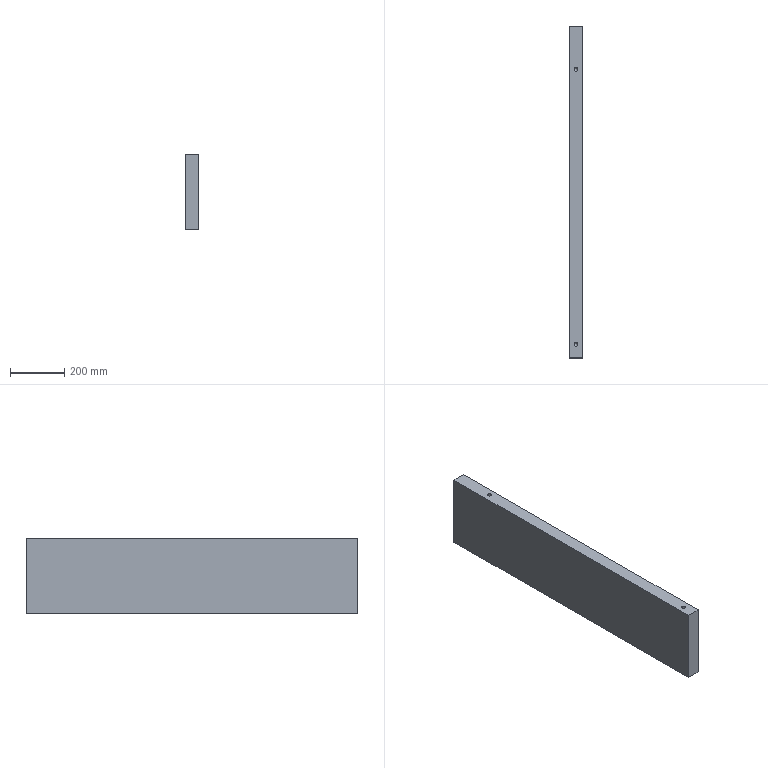Part | NX | features 29 2 | 1 solid | 16 faces | box 50 x 1225 x 280.5 mm | volume 17149943 mm3 | plane 6 | cylinder 5 | cone 5 | commonest cylinder face diameters 14.1 x5
STEP:
#1=CARTESIAN_POINT('',(2700.05,512.5,-493.5));
#2=VERTEX_POINT('',#1);
#3=CARTESIAN_POINT('',(2693.,512.5,-493.5));
#4=DIRECTION('',(0.,0.,1.));
#5=DIRECTION('',(1.,0.,0.));
#6=AXIS2_PLACEMENT_3D('',#3,#4,#5);
#7=CIRCLE('',#6,7.05);
#8=EDGE_CURVE('',#2,#2,#7,.T.);
#9=ORIENTED_EDGE('',*,*,#8,.T.);
#10=EDGE_LOOP('',(#9));
#11=FACE_BOUND('',#10,.T.);
#12=CARTESIAN_POINT('',(2668.,-552.5,-493.5));
#13=VERTEX_POINT('',#12);
#14=CARTESIAN_POINT('',(2718.,-552.5,-493.5));
#15=VERTEX_POINT('',#14);
#16=CARTESIAN_POINT('',(275.5,-552.5,-493.5));
#17=DIRECTION('',(1.,0.,0.));
#18=VECTOR('',#17,1000.);
#19=LINE('',#16,#18);
#20=EDGE_CURVE('',#13,#15,#19,.T.);
#21=ORIENTED_EDGE('',*,*,#20,.F.);
#22=CARTESIAN_POINT('',(2668.,672.5,-493.5));
#23=VERTEX_POINT('',#22);
#24=CARTESIAN_POINT('',(2668.,193.,-493.5));
#25=DIRECTION('',(0.,-1.,0.));
#26=VECTOR('',#25,1000.);
#27=LINE('',#24,#26);
#28=EDGE_CURVE('',#23,#13,#27,.T.);
#29=ORIENTED_EDGE('',*,*,#28,.F.);
#30=CARTESIAN_POINT('',(2718.,672.5,-493.5));
#31=VERTEX_POINT('',#30);
#32=CARTESIAN_POINT('',(275.5,672.5,-493.5));
#33=DIRECTION('',(1.,0.,0.));
#34=VECTOR('',#33,1000.);
#35=LINE('',#32,#34);
#36=EDGE_CURVE('',#23,#31,#35,.T.);
#37=ORIENTED_EDGE('',*,*,#36,.T.);
#38=CARTESIAN_POINT('',(2718.,193.,-493.5));
#39=DIRECTION('',(0.,1.,0.));
#40=VECTOR('',#39,1000.);
#41=LINE('',#38,#40);
#42=EDGE_CURVE('',#15,#31,#41,.T.);
#43=ORIENTED_EDGE('',*,*,#42,.F.);
#44=EDGE_LOOP('',(#21,#29,#37,#43));
#45=FACE_BOUND('',#44,.T.);
#46=CARTESIAN_POINT('',(2700.05,-502.5,-493.5));
#47=VERTEX_POINT('',#46);
#48=CARTESIAN_POINT('',(2693.,-502.5,-493.5));
#49=DIRECTION('',(0.,0.,1.));
#50=DIRECTION('',(1.,0.,0.));
#51=AXIS2_PLACEMENT_3D('',#48,#49,#50);
#52=CIRCLE('',#51,7.05);
#53=EDGE_CURVE('',#47,#47,#52,.T.);
#54=ORIENTED_EDGE('',*,*,#53,.T.);
#55=EDGE_LOOP('',(#54));
#56=FACE_BOUND('',#55,.T.);
#57=CARTESIAN_POINT('',(2700.05,60.,-493.5));
#58=VERTEX_POINT('',#57);
#59=CARTESIAN_POINT('',(2693.,60.,-493.5));
#60=DIRECTION('',(0.,0.,1.));
#61=DIRECTION('',(1.,0.,0.));
#62=AXIS2_PLACEMENT_3D('',#59,#60,#61);
#63=CIRCLE('',#62,7.05);
#64=EDGE_CURVE('',#58,#58,#63,.T.);
#65=ORIENTED_EDGE('',*,*,#64,.T.);
#66=EDGE_LOOP('',(#65));
#67=FACE_BOUND('',#66,.T.);
#68=CARTESIAN_POINT('',(2238.,0.,-493.5));
#69=DIRECTION('',(0.,0.,-1.));
#70=DIRECTION('',(1.,0.,0.));
#71=AXIS2_PLACEMENT_3D('',#68,#69,#70);
#72=PLANE('',#71);
#73=ADVANCED_FACE('',(#11,#45,#56,#67),#72,.T.);
#74=CARTESIAN_POINT('',(2700.05,512.5,-213.));
#75=VERTEX_POINT('',#74);
#76=CARTESIAN_POINT('',(2693.,512.5,-213.));
#77=DIRECTION('',(0.,0.,-1.));
#78=DIRECTION('',(1.,0.,0.));
#79=AXIS2_PLACEMENT_3D('',#76,#77,#78);
#80=CIRCLE('',#79,7.05);
#81=EDGE_CURVE('',#75,#75,#80,.T.);
#82=ORIENTED_EDGE('',*,*,#81,.T.);
#83=EDGE_LOOP('',(#82));
#84=FACE_BOUND('',#83,.T.);
#85=CARTESIAN_POINT('',(2718.,-552.5,-213.));
#86=VERTEX_POINT('',#85);
#87=CARTESIAN_POINT('',(2668.,-552.5,-213.));
#88=VERTEX_POINT('',#87);
#89=CARTESIAN_POINT('',(275.5,-552.5,-213.));
#90=DIRECTION('',(-1.,0.,0.));
#91=VECTOR('',#90,1000.);
#92=LINE('',#89,#91);
#93=EDGE_CURVE('',#86,#88,#92,.T.);
#94=ORIENTED_EDGE('',*,*,#93,.F.);
#95=CARTESIAN_POINT('',(2718.,672.5,-213.));
#96=VERTEX_POINT('',#95);
#97=CARTESIAN_POINT('',(2718.,193.,-213.));
#98=DIRECTION('',(0.,-1.,0.));
#99=VECTOR('',#98,1000.);
#100=LINE('',#97,#99);
#101=EDGE_CURVE('',#96,#86,#100,.T.);
#102=ORIENTED_EDGE('',*,*,#101,.F.);
#103=CARTESIAN_POINT('',(2668.,672.5,-213.));
#104=VERTEX_POINT('',#103);
#105=CARTESIAN_POINT('',(275.5,672.5,-213.));
#106=DIRECTION('',(-1.,0.,0.));
#107=VECTOR('',#106,1000.);
#108=LINE('',#105,#107);
#109=EDGE_CURVE('',#96,#104,#108,.T.);
#110=ORIENTED_EDGE('',*,*,#109,.T.);
#111=CARTESIAN_POINT('',(2668.,193.,-213.));
#112=DIRECTION('',(0.,1.,0.));
#113=VECTOR('',#112,1000.);
#114=LINE('',#111,#113);
#115=EDGE_CURVE('',#88,#104,#114,.T.);
#116=ORIENTED_EDGE('',*,*,#115,.F.);
#117=EDGE_LOOP('',(#94,#102,#110,#116));
#118=FACE_BOUND('',#117,.T.);
#119=CARTESIAN_POINT('',(2700.05,-502.5,-213.));
#120=VERTEX_POINT('',#119);
#121=CARTESIAN_POINT('',(2693.,-502.5,-213.));
#122=DIRECTION('',(0.,0.,-1.));
#123=DIRECTION('',(1.,0.,0.));
#124=AXIS2_PLACEMENT_3D('',#121,#122,#123);
#125=CIRCLE('',#124,7.05);
#126=EDGE_CURVE('',#120,#120,#125,.T.);
#127=ORIENTED_EDGE('',*,*,#126,.T.);
#128=EDGE_LOOP('',(#127));
#129=FACE_BOUND('',#128,.T.);
#130=CARTESIAN_POINT('',(2238.,0.,-213.));
#131=DIRECTION('',(0.,0.,1.));
#132=DIRECTION('',(-1.,0.,0.));
#133=AXIS2_PLACEMENT_3D('',#130,#131,#132);
#134=PLANE('',#133);
#135=ADVANCED_FACE('',(#84,#118,#129),#134,.T.);
#136=CARTESIAN_POINT('',(2668.,-552.5,-205.5));
#137=DIRECTION('',(0.,0.,1.));
#138=VECTOR('',#137,1000.);
#139=LINE('',#136,#138);
#140=EDGE_CURVE('',#13,#88,#139,.T.);
#141=ORIENTED_EDGE('',*,*,#140,.F.);
#142=ORIENTED_EDGE('',*,*,#20,.T.);
#143=CARTESIAN_POINT('',(2718.,-552.5,-205.5));
#144=DIRECTION('',(0.,0.,-1.));
#145=VECTOR('',#144,1000.);
#146=LINE('',#143,#145);
#147=EDGE_CURVE('',#86,#15,#146,.T.);
#148=ORIENTED_EDGE('',*,*,#147,.F.);
#149=ORIENTED_EDGE('',*,*,#93,.T.);
#150=EDGE_LOOP('',(#141,#142,#148,#149));
#151=FACE_BOUND('',#150,.T.);
#152=CARTESIAN_POINT('',(275.5,-552.5,-113.));
#153=DIRECTION('',(0.,1.,0.));
#154=DIRECTION('',(1.,0.,0.));
#155=AXIS2_PLACEMENT_3D('',#152,#153,#154);
#156=PLANE('',#155);
#157=ADVANCED_FACE('',(#151),#156,.F.);
#158=CARTESIAN_POINT('',(2668.,672.5,-205.5));
#159=DIRECTION('',(0.,0.,1.));
#160=VECTOR('',#159,1000.);
#161=LINE('',#158,#160);
#162=EDGE_CURVE('',#23,#104,#161,.T.);
#163=ORIENTED_EDGE('',*,*,#162,.F.);
#164=ORIENTED_EDGE('',*,*,#28,.T.);
#165=ORIENTED_EDGE('',*,*,#140,.T.);
#166=ORIENTED_EDGE('',*,*,#115,.T.);
#167=EDGE_LOOP('',(#163,#164,#165,#166));
#168=FACE_BOUND('',#167,.T.);
#169=CARTESIAN_POINT('',(2668.,193.,-205.5));
#170=DIRECTION('',(-1.,0.,0.));
#171=DIRECTION('',(0.,0.,1.));
#172=AXIS2_PLACEMENT_3D('',#169,#170,#171);
#173=PLANE('',#172);
#174=ADVANCED_FACE('',(#168),#173,.T.);
#175=ORIENTED_EDGE('',*,*,#147,.T.);
#176=ORIENTED_EDGE('',*,*,#42,.T.);
#177=CARTESIAN_POINT('',(2718.,672.5,91.));
#178=DIRECTION('',(0.,0.,1.));
#179=VECTOR('',#178,1000.);
#180=LINE('',#177,#179);
#181=EDGE_CURVE('',#31,#96,#180,.T.);
#182=ORIENTED_EDGE('',*,*,#181,.T.);
#183=ORIENTED_EDGE('',*,*,#101,.T.);
#184=EDGE_LOOP('',(#175,#176,#182,#183));
#185=FACE_BOUND('',#184,.T.);
#186=CARTESIAN_POINT('',(2718.,193.,-205.5));
#187=DIRECTION('',(1.,0.,0.));
#188=DIRECTION('',(0.,0.,-1.));
#189=AXIS2_PLACEMENT_3D('',#186,#187,#188);
#190=PLANE('',#189);
#191=ADVANCED_FACE('',(#185),#190,.T.);
#192=ORIENTED_EDGE('',*,*,#36,.F.);
#193=ORIENTED_EDGE('',*,*,#162,.T.);
#194=ORIENTED_EDGE('',*,*,#109,.F.);
#195=ORIENTED_EDGE('',*,*,#181,.F.);
#196=EDGE_LOOP('',(#192,#193,#194,#195));
#197=FACE_BOUND('',#196,.T.);
#198=CARTESIAN_POINT('',(275.5,672.5,91.));
#199=DIRECTION('',(0.,-1.,0.));
#200=DIRECTION('',(-1.,0.,0.));
#201=AXIS2_PLACEMENT_3D('',#198,#199,#200);
#202=PLANE('',#201);
#203=ADVANCED_FACE('',(#197),#202,.F.);
#204=CARTESIAN_POINT('',(2685.95,512.5,-249.95));
#205=VERTEX_POINT('',#204);
#206=CARTESIAN_POINT('',(2693.,512.5,-249.95));
#207=DIRECTION('',(0.,0.,-1.));
#208=DIRECTION('',(-1.,0.,0.));
#209=AXIS2_PLACEMENT_3D('',#206,#207,#208);
#210=CIRCLE('',#209,7.05);
#211=EDGE_CURVE('',#205,#205,#210,.T.);
#212=ORIENTED_EDGE('',*,*,#211,.T.);
#213=EDGE_LOOP('',(#212));
#214=FACE_BOUND('',#213,.T.);
#215=ORIENTED_EDGE('',*,*,#81,.F.);
#216=EDGE_LOOP('',(#215));
#217=FACE_BOUND('',#216,.T.);
#218=CARTESIAN_POINT('',(2693.,512.5,-213.));
#219=DIRECTION('',(0.,0.,-1.));
#220=DIRECTION('',(-1.,0.,0.));
#221=AXIS2_PLACEMENT_3D('',#218,#219,#220);
#222=CYLINDRICAL_SURFACE('',#221,7.05);
#223=ADVANCED_FACE('',(#214,#217),#222,.F.);
#224=CARTESIAN_POINT('',(2693.,512.5,-257.));
#225=VERTEX_POINT('',#224);
#226=VERTEX_LOOP('',#225);
#227=FACE_BOUND('',#226,.T.);
#228=ORIENTED_EDGE('',*,*,#211,.F.);
#229=EDGE_LOOP('',(#228));
#230=FACE_BOUND('',#229,.T.);
#231=CARTESIAN_POINT('',(2693.,512.5,-249.95));
#232=DIRECTION('',(0.,0.,1.));
#233=DIRECTION('',(-1.,0.,0.));
#234=AXIS2_PLACEMENT_3D('',#231,#232,#233);
#235=CONICAL_SURFACE('',#234,7.05,0.7854);
#236=ADVANCED_FACE('',(#227,#230),#235,.F.);
#237=CARTESIAN_POINT('',(2685.95,-502.5,-249.95));
#238=VERTEX_POINT('',#237);
#239=CARTESIAN_POINT('',(2693.,-502.5,-249.95));
#240=DIRECTION('',(0.,0.,-1.));
#241=DIRECTION('',(-1.,0.,0.));
#242=AXIS2_PLACEMENT_3D('',#239,#240,#241);
#243=CIRCLE('',#242,7.05);
#244=EDGE_CURVE('',#238,#238,#243,.T.);
#245=ORIENTED_EDGE('',*,*,#244,.T.);
#246=EDGE_LOOP('',(#245));
#247=FACE_BOUND('',#246,.T.);
#248=ORIENTED_EDGE('',*,*,#126,.F.);
#249=EDGE_LOOP('',(#248));
#250=FACE_BOUND('',#249,.T.);
#251=CARTESIAN_POINT('',(2693.,-502.5,-213.));
#252=DIRECTION('',(0.,0.,-1.));
#253=DIRECTION('',(-1.,0.,0.));
#254=AXIS2_PLACEMENT_3D('',#251,#252,#253);
#255=CYLINDRICAL_SURFACE('',#254,7.05);
#256=ADVANCED_FACE('',(#247,#250),#255,.F.);
#257=CARTESIAN_POINT('',(2693.,-502.5,-257.));
#258=VERTEX_POINT('',#257);
#259=VERTEX_LOOP('',#258);
#260=FACE_BOUND('',#259,.T.);
#261=ORIENTED_EDGE('',*,*,#244,.F.);
#262=EDGE_LOOP('',(#261));
#263=FACE_BOUND('',#262,.T.);
#264=CARTESIAN_POINT('',(2693.,-502.5,-249.95));
#265=DIRECTION('',(0.,0.,1.));
#266=DIRECTION('',(-1.,0.,0.));
#267=AXIS2_PLACEMENT_3D('',#264,#265,#266);
#268=CONICAL_SURFACE('',#267,7.05,0.7854);
#269=ADVANCED_FACE('',(#260,#263),#268,.F.);
#270=CARTESIAN_POINT('',(2700.05,-502.5,-456.55));
#271=VERTEX_POINT('',#270);
#272=CARTESIAN_POINT('',(2693.,-502.5,-456.55));
#273=DIRECTION('',(0.,0.,1.));
#274=DIRECTION('',(1.,0.,0.));
#275=AXIS2_PLACEMENT_3D('',#272,#273,#274);
#276=CIRCLE('',#275,7.05);
#277=EDGE_CURVE('',#271,#271,#276,.T.);
#278=ORIENTED_EDGE('',*,*,#277,.T.);
#279=EDGE_LOOP('',(#278));
#280=FACE_BOUND('',#279,.T.);
#281=ORIENTED_EDGE('',*,*,#53,.F.);
#282=EDGE_LOOP('',(#281));
#283=FACE_BOUND('',#282,.T.);
#284=CARTESIAN_POINT('',(2693.,-502.5,-493.5));
#285=DIRECTION('',(0.,0.,1.));
#286=DIRECTION('',(-1.,0.,0.));
#287=AXIS2_PLACEMENT_3D('',#284,#285,#286);
#288=CYLINDRICAL_SURFACE('',#287,7.05);
#289=ADVANCED_FACE('',(#280,#283),#288,.F.);
#290=CARTESIAN_POINT('',(2693.,-502.5,-449.5));
#291=VERTEX_POINT('',#290);
#292=VERTEX_LOOP('',#291);
#293=FACE_BOUND('',#292,.T.);
#294=ORIENTED_EDGE('',*,*,#277,.F.);
#295=EDGE_LOOP('',(#294));
#296=FACE_BOUND('',#295,.T.);
#297=CARTESIAN_POINT('',(2693.,-502.5,-456.55));
#298=DIRECTION('',(0.,0.,-1.));
#299=DIRECTION('',(1.,0.,0.));
#300=AXIS2_PLACEMENT_3D('',#297,#298,#299);
#301=CONICAL_SURFACE('',#300,7.05,0.7854);
#302=ADVANCED_FACE('',(#293,#296),#301,.F.);
#303=CARTESIAN_POINT('',(2700.05,512.5,-456.55));
#304=VERTEX_POINT('',#303);
#305=CARTESIAN_POINT('',(2693.,512.5,-456.55));
#306=DIRECTION('',(0.,0.,1.));
#307=DIRECTION('',(1.,0.,0.));
#308=AXIS2_PLACEMENT_3D('',#305,#306,#307);
#309=CIRCLE('',#308,7.05);
#310=EDGE_CURVE('',#304,#304,#309,.T.);
#311=ORIENTED_EDGE('',*,*,#310,.T.);
#312=EDGE_LOOP('',(#311));
#313=FACE_BOUND('',#312,.T.);
#314=ORIENTED_EDGE('',*,*,#8,.F.);
#315=EDGE_LOOP('',(#314));
#316=FACE_BOUND('',#315,.T.);
#317=CARTESIAN_POINT('',(2693.,512.5,-493.5));
#318=DIRECTION('',(0.,0.,1.));
#319=DIRECTION('',(-1.,0.,0.));
#320=AXIS2_PLACEMENT_3D('',#317,#318,#319);
#321=CYLINDRICAL_SURFACE('',#320,7.05);
#322=ADVANCED_FACE('',(#313,#316),#321,.F.);
#323=CARTESIAN_POINT('',(2693.,512.5,-449.5));
#324=VERTEX_POINT('',#323);
#325=VERTEX_LOOP('',#324);
#326=FACE_BOUND('',#325,.T.);
#327=ORIENTED_EDGE('',*,*,#310,.F.);
#328=EDGE_LOOP('',(#327));
#329=FACE_BOUND('',#328,.T.);
#330=CARTESIAN_POINT('',(2693.,512.5,-456.55));
#331=DIRECTION('',(0.,0.,-1.));
#332=DIRECTION('',(1.,0.,0.));
#333=AXIS2_PLACEMENT_3D('',#330,#331,#332);
#334=CONICAL_SURFACE('',#333,7.05,0.7854);
#335=ADVANCED_FACE('',(#326,#329),#334,.F.);
#336=CARTESIAN_POINT('',(2700.05,60.,-456.55));
#337=VERTEX_POINT('',#336);
#338=CARTESIAN_POINT('',(2693.,60.,-456.55));
#339=DIRECTION('',(0.,0.,1.));
#340=DIRECTION('',(1.,0.,0.));
#341=AXIS2_PLACEMENT_3D('',#338,#339,#340);
#342=CIRCLE('',#341,7.05);
#343=EDGE_CURVE('',#337,#337,#342,.T.);
#344=ORIENTED_EDGE('',*,*,#343,.T.);
#345=EDGE_LOOP('',(#344));
#346=FACE_BOUND('',#345,.T.);
#347=ORIENTED_EDGE('',*,*,#64,.F.);
#348=EDGE_LOOP('',(#347));
#349=FACE_BOUND('',#348,.T.);
#350=CARTESIAN_POINT('',(2693.,60.,-493.5));
#351=DIRECTION('',(0.,0.,1.));
#352=DIRECTION('',(-1.,0.,0.));
#353=AXIS2_PLACEMENT_3D('',#350,#351,#352);
#354=CYLINDRICAL_SURFACE('',#353,7.05);
#355=ADVANCED_FACE('',(#346,#349),#354,.F.);
#356=CARTESIAN_POINT('',(2693.,60.,-449.5));
#357=VERTEX_POINT('',#356);
#358=VERTEX_LOOP('',#357);
#359=FACE_BOUND('',#358,.T.);
#360=ORIENTED_EDGE('',*,*,#343,.F.);
#361=EDGE_LOOP('',(#360));
#362=FACE_BOUND('',#361,.T.);
#363=CARTESIAN_POINT('',(2693.,60.,-456.55));
#364=DIRECTION('',(0.,0.,-1.));
#365=DIRECTION('',(1.,0.,0.));
#366=AXIS2_PLACEMENT_3D('',#363,#364,#365);
#367=CONICAL_SURFACE('',#366,7.05,0.7854);
#368=ADVANCED_FACE('',(#359,#362),#367,.F.);
#369=CLOSED_SHELL('',(#73,#135,#157,#174,#191,#203,#223,#236,#256,#269,#289,#302,#322,#335,#355,#368));
#370=MANIFOLD_SOLID_BREP('',#369);
#371=(LENGTH_UNIT()NAMED_UNIT(*)SI_UNIT(.MILLI.,.METRE.));
#372=UNCERTAINTY_MEASURE_WITH_UNIT(LENGTH_MEASURE(0.00001),#371,'','');
#373=(NAMED_UNIT(*)PLANE_ANGLE_UNIT()SI_UNIT($,.RADIAN.));
#374=(NAMED_UNIT(*)SI_UNIT($,.STERADIAN.)SOLID_ANGLE_UNIT());
#375=(GEOMETRIC_REPRESENTATION_CONTEXT(3)GLOBAL_UNCERTAINTY_ASSIGNED_CONTEXT((#372))GLOBAL_UNIT_ASSIGNED_CONTEXT((#371,#373,#374))REPRESENTATION_CONTEXT('',''));
#376=ADVANCED_BREP_SHAPE_REPRESENTATION('',(#370),#375);